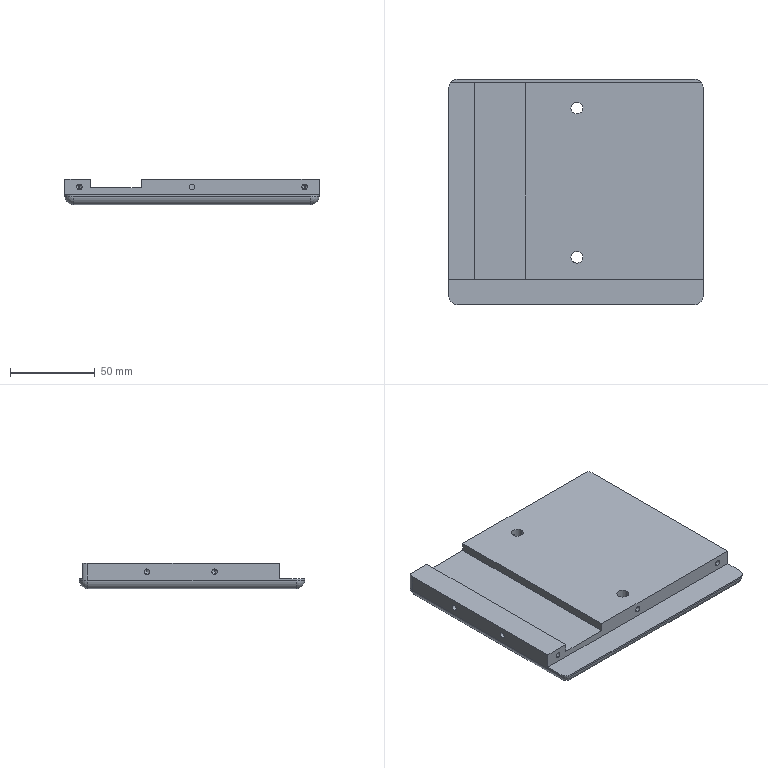Part | SolidWorks | features HoleWzd 4, ICE 3, Extrusion 1, Fillet 1, MirrorPattern 1 | 1 solid | 73 faces | box 150 x 133 x 15 mm | volume 252829 mm3 | cylinder 36 | cone 17 | plane 16 | sphere 4 | commonest cylinder face diameters 3.3 x20 10 x8 7 x4 11 x4